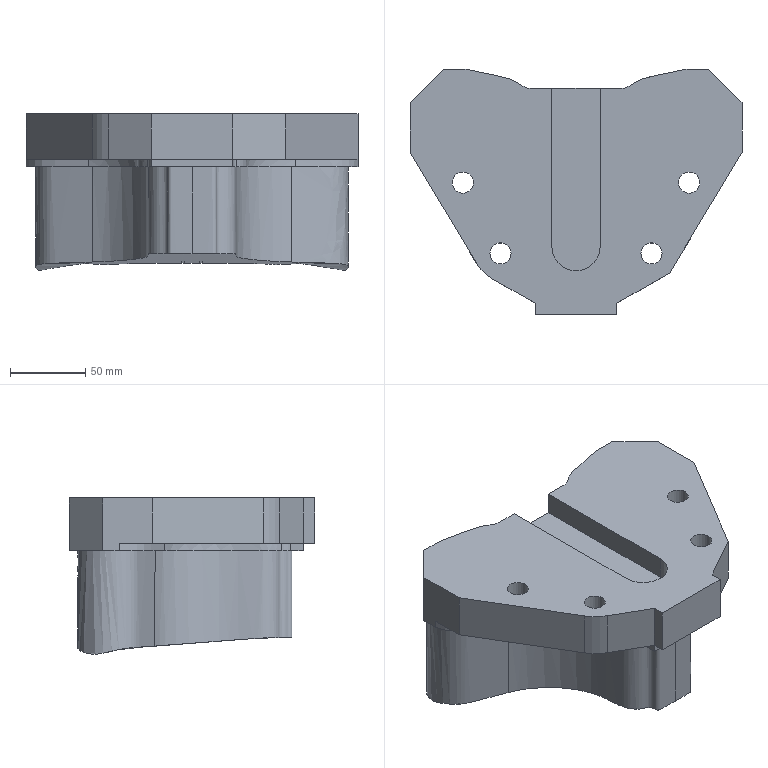Part | NX | features solid 2 | 1 solid | 125 faces | box 220 x 162.5 x 105.596 mm | volume 1671198 mm3 | spline 82 | plane 29 | cylinder 14 | commonest cylinder face diameters 14 x4 16 x4 20 x4 32 x1 60 x1